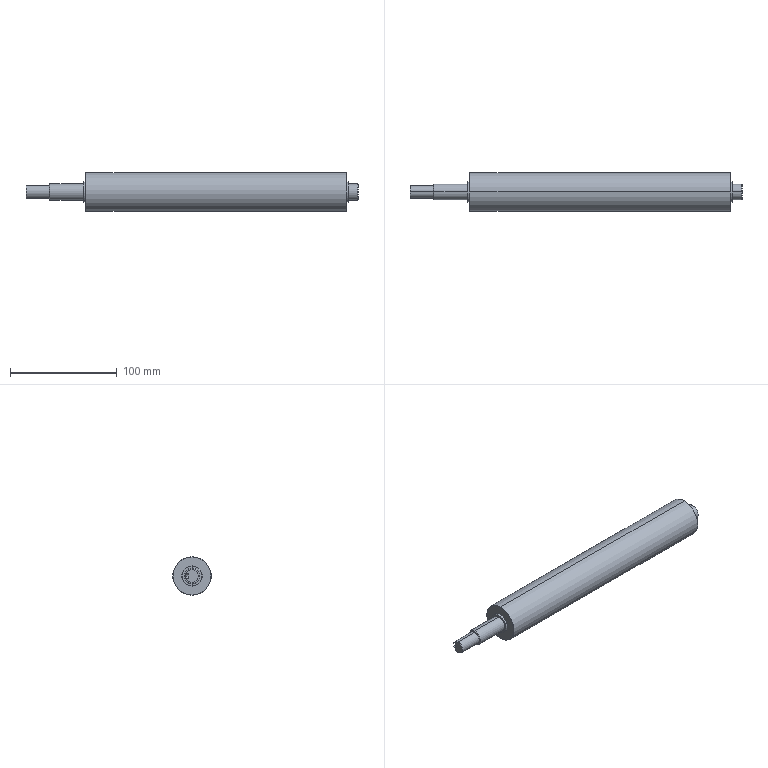Part | STEP file | 1 solid | 39 faces | box 311 x 36 x 36 mm | volume 259033 mm3 | cone 15 | cylinder 14 | plane 10 | commonest cylinder face diameters 15 x4 19 x4 4 x2 12 x2 36 x2